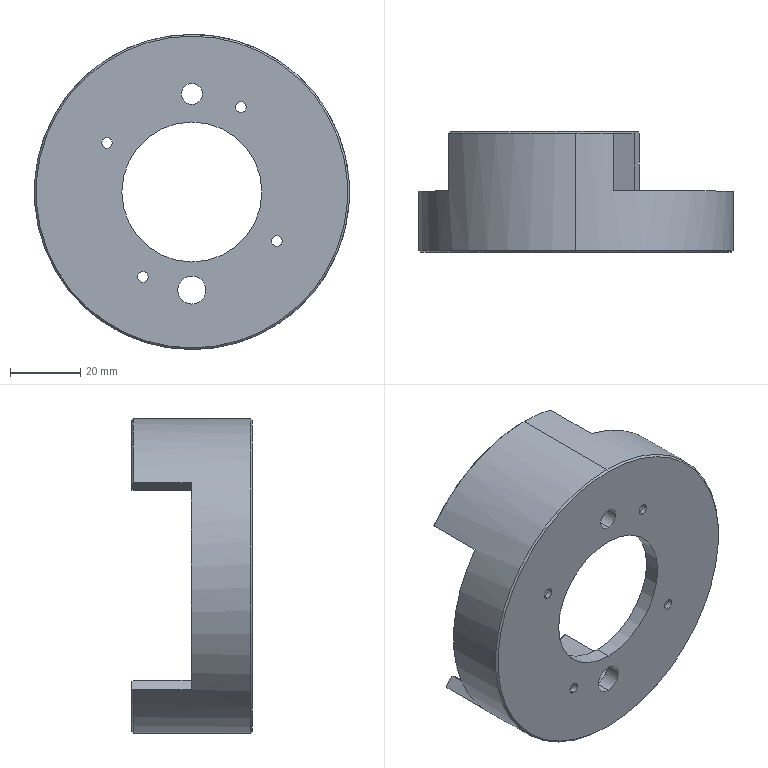Part | STEP file | PN_0017 Default | 1 solid | 52 faces | box 90 x 34.5 x 90 mm | volume 46936 mm3 | cylinder 29 | plane 13 | cone 10 | commonest cylinder face diameters 3 x8 4.5 x8 82.5 x3 6 x2 8 x2 40 x2